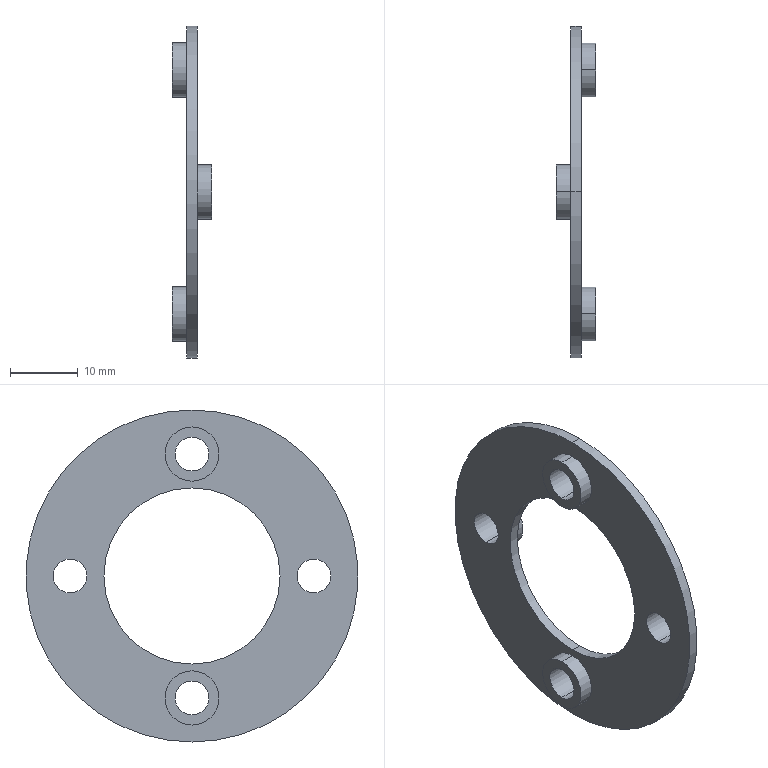Part | STEP file | _DBA01-D50-d20-e22-003 | 1 solid | 26 faces | box 5.9 x 49 x 49 mm | volume 2184 mm3 | cylinder 20 | plane 6 | commonest cylinder face diameters 5 x8 8 x8 26 x2 49 x2
STEP:
#1=CARTESIAN_POINT('',(-2.2,0.,14.));
#2=VERTEX_POINT('',#1);
#3=CARTESIAN_POINT('',(-2.2,0.,22.));
#4=VERTEX_POINT('',#3);
#5=CARTESIAN_POINT('',(-2.2,0.,18.));
#6=DIRECTION('',(-1.,0.,0.));
#7=DIRECTION('',(0.,0.,1.));
#8=AXIS2_PLACEMENT_3D('',#5,#6,#7);
#9=CIRCLE('',#8,4.);
#10=EDGE_CURVE('',#2,#4,#9,.T.);
#11=ORIENTED_EDGE('',*,*,#10,.F.);
#12=CARTESIAN_POINT('',(0.,0.,14.));
#13=VERTEX_POINT('',#12);
#14=CARTESIAN_POINT('',(-2.2,0.,14.));
#15=DIRECTION('',(1.,0.,0.));
#16=VECTOR('',#15,1000.);
#17=LINE('',#14,#16);
#18=EDGE_CURVE('',#2,#13,#17,.T.);
#19=ORIENTED_EDGE('',*,*,#18,.T.);
#20=CARTESIAN_POINT('',(0.,0.,22.));
#21=VERTEX_POINT('',#20);
#22=CARTESIAN_POINT('',(0.,0.,18.));
#23=DIRECTION('',(-1.,0.,0.));
#24=DIRECTION('',(0.,0.,1.));
#25=AXIS2_PLACEMENT_3D('',#22,#23,#24);
#26=CIRCLE('',#25,4.);
#27=EDGE_CURVE('',#13,#21,#26,.T.);
#28=ORIENTED_EDGE('',*,*,#27,.T.);
#29=CARTESIAN_POINT('',(-2.2,0.,22.));
#30=DIRECTION('',(1.,0.,0.));
#31=VECTOR('',#30,1000.);
#32=LINE('',#29,#31);
#33=EDGE_CURVE('',#4,#21,#32,.T.);
#34=ORIENTED_EDGE('',*,*,#33,.F.);
#35=EDGE_LOOP('',(#11,#19,#28,#34));
#36=FACE_OUTER_BOUND('',#35,.T.);
#37=CARTESIAN_POINT('',(-2.2,0.,18.));
#38=DIRECTION('',(1.,0.,0.));
#39=DIRECTION('',(0.,0.,1.));
#40=AXIS2_PLACEMENT_3D('',#37,#38,#39);
#41=CYLINDRICAL_SURFACE('',#40,4.);
#42=ADVANCED_FACE('',(#36),#41,.T.);
#43=CARTESIAN_POINT('',(-2.2,0.,-22.));
#44=VERTEX_POINT('',#43);
#45=CARTESIAN_POINT('',(-2.2,0.,-14.));
#46=VERTEX_POINT('',#45);
#47=CARTESIAN_POINT('',(-2.2,0.,-18.));
#48=DIRECTION('',(-1.,0.,0.));
#49=DIRECTION('',(0.,0.,1.));
#50=AXIS2_PLACEMENT_3D('',#47,#48,#49);
#51=CIRCLE('',#50,4.);
#52=EDGE_CURVE('',#44,#46,#51,.T.);
#53=ORIENTED_EDGE('',*,*,#52,.F.);
#54=CARTESIAN_POINT('',(0.,0.,-22.));
#55=VERTEX_POINT('',#54);
#56=CARTESIAN_POINT('',(-2.2,0.,-22.));
#57=DIRECTION('',(1.,0.,0.));
#58=VECTOR('',#57,1000.);
#59=LINE('',#56,#58);
#60=EDGE_CURVE('',#44,#55,#59,.T.);
#61=ORIENTED_EDGE('',*,*,#60,.T.);
#62=CARTESIAN_POINT('',(0.,0.,-14.));
#63=VERTEX_POINT('',#62);
#64=CARTESIAN_POINT('',(0.,0.,-18.));
#65=DIRECTION('',(-1.,0.,0.));
#66=DIRECTION('',(0.,0.,1.));
#67=AXIS2_PLACEMENT_3D('',#64,#65,#66);
#68=CIRCLE('',#67,4.);
#69=EDGE_CURVE('',#55,#63,#68,.T.);
#70=ORIENTED_EDGE('',*,*,#69,.T.);
#71=CARTESIAN_POINT('',(-2.2,0.,-14.));
#72=DIRECTION('',(1.,0.,0.));
#73=VECTOR('',#72,1000.);
#74=LINE('',#71,#73);
#75=EDGE_CURVE('',#46,#63,#74,.T.);
#76=ORIENTED_EDGE('',*,*,#75,.F.);
#77=EDGE_LOOP('',(#53,#61,#70,#76));
#78=FACE_OUTER_BOUND('',#77,.T.);
#79=CARTESIAN_POINT('',(-2.2,0.,-18.));
#80=DIRECTION('',(1.,0.,0.));
#81=DIRECTION('',(0.,0.,1.));
#82=AXIS2_PLACEMENT_3D('',#79,#80,#81);
#83=CYLINDRICAL_SURFACE('',#82,4.);
#84=ADVANCED_FACE('',(#78),#83,.T.);
#85=CARTESIAN_POINT('',(1.5,-18.,4.));
#86=VERTEX_POINT('',#85);
#87=CARTESIAN_POINT('',(1.5,-18.,-4.));
#88=VERTEX_POINT('',#87);
#89=CARTESIAN_POINT('',(1.5,-18.,0.));
#90=DIRECTION('',(1.,0.,0.));
#91=DIRECTION('',(0.,0.,-1.));
#92=AXIS2_PLACEMENT_3D('',#89,#90,#91);
#93=CIRCLE('',#92,4.);
#94=EDGE_CURVE('',#86,#88,#93,.T.);
#95=ORIENTED_EDGE('',*,*,#94,.T.);
#96=CARTESIAN_POINT('',(3.7,-18.,-4.));
#97=VERTEX_POINT('',#96);
#98=CARTESIAN_POINT('',(1.5,-18.,-4.));
#99=DIRECTION('',(1.,0.,0.));
#100=VECTOR('',#99,1000.);
#101=LINE('',#98,#100);
#102=EDGE_CURVE('',#88,#97,#101,.T.);
#103=ORIENTED_EDGE('',*,*,#102,.T.);
#104=CARTESIAN_POINT('',(3.7,-18.,4.));
#105=VERTEX_POINT('',#104);
#106=CARTESIAN_POINT('',(3.7,-18.,0.));
#107=DIRECTION('',(-1.,0.,0.));
#108=DIRECTION('',(0.,0.,1.));
#109=AXIS2_PLACEMENT_3D('',#106,#107,#108);
#110=CIRCLE('',#109,4.);
#111=EDGE_CURVE('',#97,#105,#110,.T.);
#112=ORIENTED_EDGE('',*,*,#111,.T.);
#113=CARTESIAN_POINT('',(1.5,-18.,4.));
#114=DIRECTION('',(1.,0.,0.));
#115=VECTOR('',#114,1000.);
#116=LINE('',#113,#115);
#117=EDGE_CURVE('',#86,#105,#116,.T.);
#118=ORIENTED_EDGE('',*,*,#117,.F.);
#119=EDGE_LOOP('',(#95,#103,#112,#118));
#120=FACE_OUTER_BOUND('',#119,.T.);
#121=CARTESIAN_POINT('',(1.5,-18.,0.));
#122=DIRECTION('',(1.,0.,0.));
#123=DIRECTION('',(0.,0.,1.));
#124=AXIS2_PLACEMENT_3D('',#121,#122,#123);
#125=CYLINDRICAL_SURFACE('',#124,4.);
#126=ADVANCED_FACE('',(#120),#125,.T.);
#127=CARTESIAN_POINT('',(1.5,18.,4.));
#128=VERTEX_POINT('',#127);
#129=CARTESIAN_POINT('',(1.5,18.,-4.));
#130=VERTEX_POINT('',#129);
#131=CARTESIAN_POINT('',(1.5,18.,0.));
#132=DIRECTION('',(1.,0.,0.));
#133=DIRECTION('',(0.,0.,-1.));
#134=AXIS2_PLACEMENT_3D('',#131,#132,#133);
#135=CIRCLE('',#134,4.);
#136=EDGE_CURVE('',#128,#130,#135,.T.);
#137=ORIENTED_EDGE('',*,*,#136,.T.);
#138=CARTESIAN_POINT('',(3.7,18.,-4.));
#139=VERTEX_POINT('',#138);
#140=CARTESIAN_POINT('',(1.5,18.,-4.));
#141=DIRECTION('',(1.,0.,0.));
#142=VECTOR('',#141,1000.);
#143=LINE('',#140,#142);
#144=EDGE_CURVE('',#130,#139,#143,.T.);
#145=ORIENTED_EDGE('',*,*,#144,.T.);
#146=CARTESIAN_POINT('',(3.7,18.,4.));
#147=VERTEX_POINT('',#146);
#148=CARTESIAN_POINT('',(3.7,18.,0.));
#149=DIRECTION('',(-1.,0.,0.));
#150=DIRECTION('',(0.,0.,1.));
#151=AXIS2_PLACEMENT_3D('',#148,#149,#150);
#152=CIRCLE('',#151,4.);
#153=EDGE_CURVE('',#139,#147,#152,.T.);
#154=ORIENTED_EDGE('',*,*,#153,.T.);
#155=CARTESIAN_POINT('',(1.5,18.,4.));
#156=DIRECTION('',(1.,0.,0.));
#157=VECTOR('',#156,1000.);
#158=LINE('',#155,#157);
#159=EDGE_CURVE('',#128,#147,#158,.T.);
#160=ORIENTED_EDGE('',*,*,#159,.F.);
#161=EDGE_LOOP('',(#137,#145,#154,#160));
#162=FACE_OUTER_BOUND('',#161,.T.);
#163=CARTESIAN_POINT('',(1.5,18.,0.));
#164=DIRECTION('',(1.,0.,0.));
#165=DIRECTION('',(0.,0.,1.));
#166=AXIS2_PLACEMENT_3D('',#163,#164,#165);
#167=CYLINDRICAL_SURFACE('',#166,4.);
#168=ADVANCED_FACE('',(#162),#167,.T.);
#169=CARTESIAN_POINT('',(-2.2,0.,-15.5));
#170=VERTEX_POINT('',#169);
#171=CARTESIAN_POINT('',(-2.2,0.,-20.5));
#172=VERTEX_POINT('',#171);
#173=CARTESIAN_POINT('',(-2.2,0.,-18.));
#174=DIRECTION('',(-1.,0.,0.));
#175=DIRECTION('',(0.,0.,1.));
#176=AXIS2_PLACEMENT_3D('',#173,#174,#175);
#177=CIRCLE('',#176,2.5);
#178=EDGE_CURVE('',#170,#172,#177,.T.);
#179=ORIENTED_EDGE('',*,*,#178,.T.);
#180=CARTESIAN_POINT('',(1.5,0.,-20.5));
#181=VERTEX_POINT('',#180);
#182=CARTESIAN_POINT('',(1.5,0.,-20.5));
#183=DIRECTION('',(1.,0.,0.));
#184=VECTOR('',#183,1000.);
#185=LINE('',#182,#184);
#186=EDGE_CURVE('',#172,#181,#185,.T.);
#187=ORIENTED_EDGE('',*,*,#186,.T.);
#188=CARTESIAN_POINT('',(1.5,0.,-15.5));
#189=VERTEX_POINT('',#188);
#190=CARTESIAN_POINT('',(1.5,0.,-18.));
#191=DIRECTION('',(1.,0.,0.));
#192=DIRECTION('',(0.,0.,-1.));
#193=AXIS2_PLACEMENT_3D('',#190,#191,#192);
#194=CIRCLE('',#193,2.5);
#195=EDGE_CURVE('',#181,#189,#194,.T.);
#196=ORIENTED_EDGE('',*,*,#195,.T.);
#197=CARTESIAN_POINT('',(1.5,0.,-15.5));
#198=DIRECTION('',(1.,0.,0.));
#199=VECTOR('',#198,1000.);
#200=LINE('',#197,#199);
#201=EDGE_CURVE('',#170,#189,#200,.T.);
#202=ORIENTED_EDGE('',*,*,#201,.F.);
#203=EDGE_LOOP('',(#179,#187,#196,#202));
#204=FACE_OUTER_BOUND('',#203,.T.);
#205=CARTESIAN_POINT('',(1.5,0.,-18.));
#206=DIRECTION('',(1.,0.,0.));
#207=DIRECTION('',(0.,0.,1.));
#208=AXIS2_PLACEMENT_3D('',#205,#206,#207);
#209=CYLINDRICAL_SURFACE('',#208,2.5);
#210=ADVANCED_FACE('',(#204),#209,.F.);
#211=CARTESIAN_POINT('',(0.,-18.,2.5));
#212=VERTEX_POINT('',#211);
#213=CARTESIAN_POINT('',(0.,-18.,-2.5));
#214=VERTEX_POINT('',#213);
#215=CARTESIAN_POINT('',(0.,-18.,0.));
#216=DIRECTION('',(-1.,0.,0.));
#217=DIRECTION('',(0.,0.,-1.));
#218=AXIS2_PLACEMENT_3D('',#215,#216,#217);
#219=CIRCLE('',#218,2.5);
#220=EDGE_CURVE('',#212,#214,#219,.T.);
#221=ORIENTED_EDGE('',*,*,#220,.T.);
#222=CARTESIAN_POINT('',(3.7,-18.,-2.5));
#223=VERTEX_POINT('',#222);
#224=CARTESIAN_POINT('',(1.5,-18.,-2.5));
#225=DIRECTION('',(1.,0.,0.));
#226=VECTOR('',#225,1000.);
#227=LINE('',#224,#226);
#228=EDGE_CURVE('',#214,#223,#227,.T.);
#229=ORIENTED_EDGE('',*,*,#228,.T.);
#230=CARTESIAN_POINT('',(3.7,-18.,2.5));
#231=VERTEX_POINT('',#230);
#232=CARTESIAN_POINT('',(3.7,-18.,0.));
#233=DIRECTION('',(-1.,0.,0.));
#234=DIRECTION('',(0.,0.,1.));
#235=AXIS2_PLACEMENT_3D('',#232,#233,#234);
#236=CIRCLE('',#235,2.5);
#237=EDGE_CURVE('',#231,#223,#236,.T.);
#238=ORIENTED_EDGE('',*,*,#237,.F.);
#239=CARTESIAN_POINT('',(1.5,-18.,2.5));
#240=DIRECTION('',(1.,0.,0.));
#241=VECTOR('',#240,1000.);
#242=LINE('',#239,#241);
#243=EDGE_CURVE('',#212,#231,#242,.T.);
#244=ORIENTED_EDGE('',*,*,#243,.F.);
#245=EDGE_LOOP('',(#221,#229,#238,#244));
#246=FACE_OUTER_BOUND('',#245,.T.);
#247=CARTESIAN_POINT('',(1.5,-18.,0.));
#248=DIRECTION('',(1.,0.,0.));
#249=DIRECTION('',(0.,0.,1.));
#250=AXIS2_PLACEMENT_3D('',#247,#248,#249);
#251=CYLINDRICAL_SURFACE('',#250,2.5);
#252=ADVANCED_FACE('',(#246),#251,.F.);
#253=CARTESIAN_POINT('',(-2.2,0.,20.5));
#254=VERTEX_POINT('',#253);
#255=CARTESIAN_POINT('',(-2.2,0.,15.5));
#256=VERTEX_POINT('',#255);
#257=CARTESIAN_POINT('',(-2.2,0.,18.));
#258=DIRECTION('',(-1.,0.,0.));
#259=DIRECTION('',(0.,0.,1.));
#260=AXIS2_PLACEMENT_3D('',#257,#258,#259);
#261=CIRCLE('',#260,2.5);
#262=EDGE_CURVE('',#254,#256,#261,.T.);
#263=ORIENTED_EDGE('',*,*,#262,.T.);
#264=CARTESIAN_POINT('',(1.5,0.,15.5));
#265=VERTEX_POINT('',#264);
#266=CARTESIAN_POINT('',(1.5,0.,15.5));
#267=DIRECTION('',(1.,0.,0.));
#268=VECTOR('',#267,1000.);
#269=LINE('',#266,#268);
#270=EDGE_CURVE('',#256,#265,#269,.T.);
#271=ORIENTED_EDGE('',*,*,#270,.T.);
#272=CARTESIAN_POINT('',(1.5,0.,20.5));
#273=VERTEX_POINT('',#272);
#274=CARTESIAN_POINT('',(1.5,0.,18.));
#275=DIRECTION('',(1.,0.,0.));
#276=DIRECTION('',(0.,0.,-1.));
#277=AXIS2_PLACEMENT_3D('',#274,#275,#276);
#278=CIRCLE('',#277,2.5);
#279=EDGE_CURVE('',#265,#273,#278,.T.);
#280=ORIENTED_EDGE('',*,*,#279,.T.);
#281=CARTESIAN_POINT('',(1.5,0.,20.5));
#282=DIRECTION('',(1.,0.,0.));
#283=VECTOR('',#282,1000.);
#284=LINE('',#281,#283);
#285=EDGE_CURVE('',#254,#273,#284,.T.);
#286=ORIENTED_EDGE('',*,*,#285,.F.);
#287=EDGE_LOOP('',(#263,#271,#280,#286));
#288=FACE_OUTER_BOUND('',#287,.T.);
#289=CARTESIAN_POINT('',(1.5,0.,18.));
#290=DIRECTION('',(1.,0.,0.));
#291=DIRECTION('',(0.,0.,1.));
#292=AXIS2_PLACEMENT_3D('',#289,#290,#291);
#293=CYLINDRICAL_SURFACE('',#292,2.5);
#294=ADVANCED_FACE('',(#288),#293,.F.);
#295=CARTESIAN_POINT('',(0.,18.,2.5));
#296=VERTEX_POINT('',#295);
#297=CARTESIAN_POINT('',(0.,18.,-2.5));
#298=VERTEX_POINT('',#297);
#299=CARTESIAN_POINT('',(0.,18.,0.));
#300=DIRECTION('',(-1.,0.,0.));
#301=DIRECTION('',(0.,0.,-1.));
#302=AXIS2_PLACEMENT_3D('',#299,#300,#301);
#303=CIRCLE('',#302,2.5);
#304=EDGE_CURVE('',#296,#298,#303,.T.);
#305=ORIENTED_EDGE('',*,*,#304,.T.);
#306=CARTESIAN_POINT('',(3.7,18.,-2.5));
#307=VERTEX_POINT('',#306);
#308=CARTESIAN_POINT('',(1.5,18.,-2.5));
#309=DIRECTION('',(1.,0.,0.));
#310=VECTOR('',#309,1000.);
#311=LINE('',#308,#310);
#312=EDGE_CURVE('',#298,#307,#311,.T.);
#313=ORIENTED_EDGE('',*,*,#312,.T.);
#314=CARTESIAN_POINT('',(3.7,18.,2.5));
#315=VERTEX_POINT('',#314);
#316=CARTESIAN_POINT('',(3.7,18.,0.));
#317=DIRECTION('',(-1.,0.,0.));
#318=DIRECTION('',(0.,0.,1.));
#319=AXIS2_PLACEMENT_3D('',#316,#317,#318);
#320=CIRCLE('',#319,2.5);
#321=EDGE_CURVE('',#315,#307,#320,.T.);
#322=ORIENTED_EDGE('',*,*,#321,.F.);
#323=CARTESIAN_POINT('',(1.5,18.,2.5));
#324=DIRECTION('',(1.,0.,0.));
#325=VECTOR('',#324,1000.);
#326=LINE('',#323,#325);
#327=EDGE_CURVE('',#296,#315,#326,.T.);
#328=ORIENTED_EDGE('',*,*,#327,.F.);
#329=EDGE_LOOP('',(#305,#313,#322,#328));
#330=FACE_OUTER_BOUND('',#329,.T.);
#331=CARTESIAN_POINT('',(1.5,18.,0.));
#332=DIRECTION('',(1.,0.,0.));
#333=DIRECTION('',(0.,0.,1.));
#334=AXIS2_PLACEMENT_3D('',#331,#332,#333);
#335=CYLINDRICAL_SURFACE('',#334,2.5);
#336=ADVANCED_FACE('',(#330),#335,.F.);
#337=CARTESIAN_POINT('',(0.,0.,-13.));
#338=VERTEX_POINT('',#337);
#339=CARTESIAN_POINT('',(0.,0.,13.));
#340=VERTEX_POINT('',#339);
#341=CARTESIAN_POINT('',(0.,0.,0.));
#342=DIRECTION('',(1.,0.,0.));
#343=DIRECTION('',(0.,0.,-1.));
#344=AXIS2_PLACEMENT_3D('',#341,#342,#343);
#345=CIRCLE('',#344,13.);
#346=EDGE_CURVE('',#338,#340,#345,.T.);
#347=ORIENTED_EDGE('',*,*,#346,.F.);
#348=CARTESIAN_POINT('',(1.5,0.,-13.));
#349=VERTEX_POINT('',#348);
#350=CARTESIAN_POINT('',(1.5,0.,-13.));
#351=DIRECTION('',(1.,0.,0.));
#352=VECTOR('',#351,1000.);
#353=LINE('',#350,#352);
#354=EDGE_CURVE('',#338,#349,#353,.T.);
#355=ORIENTED_EDGE('',*,*,#354,.T.);
#356=CARTESIAN_POINT('',(1.5,0.,13.));
#357=VERTEX_POINT('',#356);
#358=CARTESIAN_POINT('',(1.5,0.,0.));
#359=DIRECTION('',(1.,0.,0.));
#360=DIRECTION('',(0.,0.,-1.));
#361=AXIS2_PLACEMENT_3D('',#358,#359,#360);
#362=CIRCLE('',#361,13.);
#363=EDGE_CURVE('',#349,#357,#362,.T.);
#364=ORIENTED_EDGE('',*,*,#363,.T.);
#365=CARTESIAN_POINT('',(1.5,0.,13.));
#366=DIRECTION('',(1.,0.,0.));
#367=VECTOR('',#366,1000.);
#368=LINE('',#365,#367);
#369=EDGE_CURVE('',#340,#357,#368,.T.);
#370=ORIENTED_EDGE('',*,*,#369,.F.);
#371=EDGE_LOOP('',(#347,#355,#364,#370));
#372=FACE_OUTER_BOUND('',#371,.T.);
#373=CARTESIAN_POINT('',(1.5,0.,0.));
#374=DIRECTION('',(1.,0.,0.));
#375=DIRECTION('',(0.,0.,1.));
#376=AXIS2_PLACEMENT_3D('',#373,#374,#375);
#377=CYLINDRICAL_SURFACE('',#376,13.);
#378=ADVANCED_FACE('',(#372),#377,.F.);
#379=CARTESIAN_POINT('',(0.,0.,24.5));
#380=VERTEX_POINT('',#379);
#381=CARTESIAN_POINT('',(0.,0.,-24.5));
#382=VERTEX_POINT('',#381);
#383=CARTESIAN_POINT('',(0.,0.,0.));
#384=DIRECTION('',(1.,0.,0.));
#385=DIRECTION('',(0.,0.,-1.));
#386=AXIS2_PLACEMENT_3D('',#383,#384,#385);
#387=CIRCLE('',#386,24.5);
#388=EDGE_CURVE('',#380,#382,#387,.T.);
#389=ORIENTED_EDGE('',*,*,#388,.T.);
#390=CARTESIAN_POINT('',(1.5,0.,-24.5));
#391=VERTEX_POINT('',#390);
#392=CARTESIAN_POINT('',(1.5,0.,-24.5));
#393=DIRECTION('',(1.,0.,0.));
#394=VECTOR('',#393,1000.);
#395=LINE('',#392,#394);
#396=EDGE_CURVE('',#382,#391,#395,.T.);
#397=ORIENTED_EDGE('',*,*,#396,.T.);
#398=CARTESIAN_POINT('',(1.5,0.,24.5));
#399=VERTEX_POINT('',#398);
#400=CARTESIAN_POINT('',(1.5,0.,0.));
#401=DIRECTION('',(1.,0.,0.));
#402=DIRECTION('',(0.,0.,-1.));
#403=AXIS2_PLACEMENT_3D('',#400,#401,#402);
#404=CIRCLE('',#403,24.5);
#405=EDGE_CURVE('',#399,#391,#404,.T.);
#406=ORIENTED_EDGE('',*,*,#405,.F.);
#407=CARTESIAN_POINT('',(1.5,0.,24.5));
#408=DIRECTION('',(1.,0.,0.));
#409=VECTOR('',#408,1000.);
#410=LINE('',#407,#409);
#411=EDGE_CURVE('',#380,#399,#410,.T.);
#412=ORIENTED_EDGE('',*,*,#411,.F.);
#413=EDGE_LOOP('',(#389,#397,#406,#412));
#414=FACE_OUTER_BOUND('',#413,.T.);
#415=CARTESIAN_POINT('',(1.5,0.,0.));
#416=DIRECTION('',(1.,0.,0.));
#417=DIRECTION('',(0.,0.,1.));
#418=AXIS2_PLACEMENT_3D('',#415,#416,#417);
#419=CYLINDRICAL_SURFACE('',#418,24.5);
#420=ADVANCED_FACE('',(#414),#419,.T.);
#421=ORIENTED_EDGE('',*,*,#388,.F.);
#422=CARTESIAN_POINT('',(0.,0.,0.));
#423=DIRECTION('',(1.,0.,0.));
#424=DIRECTION('',(0.,0.,-1.));
#425=AXIS2_PLACEMENT_3D('',#422,#423,#424);
#426=CIRCLE('',#425,24.5);
#427=EDGE_CURVE('',#382,#380,#426,.T.);
#428=ORIENTED_EDGE('',*,*,#427,.F.);
#429=EDGE_LOOP('',(#421,#428));
#430=FACE_OUTER_BOUND('',#429,.T.);
#431=CARTESIAN_POINT('',(0.,0.,18.));
#432=DIRECTION('',(-1.,0.,0.));
#433=DIRECTION('',(0.,0.,1.));
#434=AXIS2_PLACEMENT_3D('',#431,#432,#433);
#435=CIRCLE('',#434,4.);
#436=EDGE_CURVE('',#21,#13,#435,.T.);
#437=ORIENTED_EDGE('',*,*,#436,.F.);
#438=ORIENTED_EDGE('',*,*,#27,.F.);
#439=EDGE_LOOP('',(#437,#438));
#440=FACE_BOUND('',#439,.T.);
#441=CARTESIAN_POINT('',(0.,0.,-18.));
#442=DIRECTION('',(-1.,0.,0.));
#443=DIRECTION('',(0.,0.,1.));
#444=AXIS2_PLACEMENT_3D('',#441,#442,#443);
#445=CIRCLE('',#444,4.);
#446=EDGE_CURVE('',#63,#55,#445,.T.);
#447=ORIENTED_EDGE('',*,*,#446,.F.);
#448=ORIENTED_EDGE('',*,*,#69,.F.);
#449=EDGE_LOOP('',(#447,#448));
#450=FACE_BOUND('',#449,.T.);
#451=ORIENTED_EDGE('',*,*,#220,.F.);
#452=CARTESIAN_POINT('',(0.,-18.,0.));
#453=DIRECTION('',(-1.,0.,0.));
#454=DIRECTION('',(0.,0.,-1.));
#455=AXIS2_PLACEMENT_3D('',#452,#453,#454);
#456=CIRCLE('',#455,2.5);
#457=EDGE_CURVE('',#214,#212,#456,.T.);
#458=ORIENTED_EDGE('',*,*,#457,.F.);
#459=EDGE_LOOP('',(#451,#458));
#460=FACE_BOUND('',#459,.T.);
#461=ORIENTED_EDGE('',*,*,#304,.F.);
#462=CARTESIAN_POINT('',(0.,18.,0.));
#463=DIRECTION('',(-1.,0.,0.));
#464=DIRECTION('',(0.,0.,-1.));
#465=AXIS2_PLACEMENT_3D('',#462,#463,#464);
#466=CIRCLE('',#465,2.5);
#467=EDGE_CURVE('',#298,#296,#466,.T.);
#468=ORIENTED_EDGE('',*,*,#467,.F.);
#469=EDGE_LOOP('',(#461,#468));
#470=FACE_BOUND('',#469,.T.);
#471=CARTESIAN_POINT('',(0.,0.,0.));
#472=DIRECTION('',(1.,0.,0.));
#473=DIRECTION('',(0.,0.,-1.));
#474=AXIS2_PLACEMENT_3D('',#471,#472,#473);
#475=CIRCLE('',#474,13.);
#476=EDGE_CURVE('',#340,#338,#475,.T.);
#477=ORIENTED_EDGE('',*,*,#476,.T.);
#478=ORIENTED_EDGE('',*,*,#346,.T.);
#479=EDGE_LOOP('',(#477,#478));
#480=FACE_BOUND('',#479,.T.);
#481=CARTESIAN_POINT('',(0.,0.,0.));
#482=DIRECTION('',(1.,0.,0.));
#483=DIRECTION('',(0.,1.,0.));
#484=AXIS2_PLACEMENT_3D('',#481,#482,#483);
#485=PLANE('',#484);
#486=ADVANCED_FACE('',(#430,#440,#450,#460,#470,#480),#485,.F.);
#487=ORIENTED_EDGE('',*,*,#396,.F.);
#488=ORIENTED_EDGE('',*,*,#427,.T.);
#489=ORIENTED_EDGE('',*,*,#411,.T.);
#490=CARTESIAN_POINT('',(1.5,0.,0.));
#491=DIRECTION('',(1.,0.,0.));
#492=DIRECTION('',(0.,0.,-1.));
#493=AXIS2_PLACEMENT_3D('',#490,#491,#492);
#494=CIRCLE('',#493,24.5);
#495=EDGE_CURVE('',#391,#399,#494,.T.);
#496=ORIENTED_EDGE('',*,*,#495,.F.);
#497=EDGE_LOOP('',(#487,#488,#489,#496));
#498=FACE_OUTER_BOUND('',#497,.T.);
#499=CARTESIAN_POINT('',(1.5,0.,0.));
#500=DIRECTION('',(1.,0.,0.));
#501=DIRECTION('',(0.,0.,1.));
#502=AXIS2_PLACEMENT_3D('',#499,#500,#501);
#503=CYLINDRICAL_SURFACE('',#502,24.5);
#504=ADVANCED_FACE('',(#498),#503,.T.);
#505=ORIENTED_EDGE('',*,*,#405,.T.);
#506=ORIENTED_EDGE('',*,*,#495,.T.);
#507=EDGE_LOOP('',(#505,#506));
#508=FACE_OUTER_BOUND('',#507,.T.);
#509=ORIENTED_EDGE('',*,*,#94,.F.);
#510=CARTESIAN_POINT('',(1.5,-18.,0.));
#511=DIRECTION('',(1.,0.,0.));
#512=DIRECTION('',(0.,0.,-1.));
#513=AXIS2_PLACEMENT_3D('',#510,#511,#512);
#514=CIRCLE('',#513,4.);
#515=EDGE_CURVE('',#88,#86,#514,.T.);
#516=ORIENTED_EDGE('',*,*,#515,.F.);
#517=EDGE_LOOP('',(#509,#516));
#518=FACE_BOUND('',#517,.T.);
#519=ORIENTED_EDGE('',*,*,#136,.F.);
#520=CARTESIAN_POINT('',(1.5,18.,0.));
#521=DIRECTION('',(1.,0.,0.));
#522=DIRECTION('',(0.,0.,-1.));
#523=AXIS2_PLACEMENT_3D('',#520,#521,#522);
#524=CIRCLE('',#523,4.);
#525=EDGE_CURVE('',#130,#128,#524,.T.);
#526=ORIENTED_EDGE('',*,*,#525,.F.);
#527=EDGE_LOOP('',(#519,#526));
#528=FACE_BOUND('',#527,.T.);
#529=CARTESIAN_POINT('',(1.5,0.,-18.));
#530=DIRECTION('',(1.,0.,0.));
#531=DIRECTION('',(0.,0.,-1.));
#532=AXIS2_PLACEMENT_3D('',#529,#530,#531);
#533=CIRCLE('',#532,2.5);
#534=EDGE_CURVE('',#189,#181,#533,.T.);
#535=ORIENTED_EDGE('',*,*,#534,.F.);
#536=ORIENTED_EDGE('',*,*,#195,.F.);
#537=EDGE_LOOP('',(#535,#536));
#538=FACE_BOUND('',#537,.T.);
#539=CARTESIAN_POINT('',(1.5,0.,18.));
#540=DIRECTION('',(1.,0.,0.));
#541=DIRECTION('',(0.,0.,-1.));
#542=AXIS2_PLACEMENT_3D('',#539,#540,#541);
#543=CIRCLE('',#542,2.5);
#544=EDGE_CURVE('',#273,#265,#543,.T.);
#545=ORIENTED_EDGE('',*,*,#544,.F.);
#546=ORIENTED_EDGE('',*,*,#279,.F.);
#547=EDGE_LOOP('',(#545,#546));
#548=FACE_BOUND('',#547,.T.);
#549=CARTESIAN_POINT('',(1.5,0.,0.));
#550=DIRECTION('',(1.,0.,0.));
#551=DIRECTION('',(0.,0.,-1.));
#552=AXIS2_PLACEMENT_3D('',#549,#550,#551);
#553=CIRCLE('',#552,13.);
#554=EDGE_CURVE('',#357,#349,#553,.T.);
#555=ORIENTED_EDGE('',*,*,#554,.F.);
#556=ORIENTED_EDGE('',*,*,#363,.F.);
#557=EDGE_LOOP('',(#555,#556));
#558=FACE_BOUND('',#557,.T.);
#559=CARTESIAN_POINT('',(1.5,0.,0.));
#560=DIRECTION('',(1.,0.,0.));
#561=DIRECTION('',(0.,1.,0.));
#562=AXIS2_PLACEMENT_3D('',#559,#560,#561);
#563=PLANE('',#562);
#564=ADVANCED_FACE('',(#508,#518,#528,#538,#548,#558),#563,.T.);
#565=ORIENTED_EDGE('',*,*,#354,.F.);
#566=ORIENTED_EDGE('',*,*,#476,.F.);
#567=ORIENTED_EDGE('',*,*,#369,.T.);
#568=ORIENTED_EDGE('',*,*,#554,.T.);
#569=EDGE_LOOP('',(#565,#566,#567,#568));
#570=FACE_OUTER_BOUND('',#569,.T.);
#571=CARTESIAN_POINT('',(1.5,0.,0.));
#572=DIRECTION('',(1.,0.,0.));
#573=DIRECTION('',(0.,0.,1.));
#574=AXIS2_PLACEMENT_3D('',#571,#572,#573);
#575=CYLINDRICAL_SURFACE('',#574,13.);
#576=ADVANCED_FACE('',(#570),#575,.F.);
#577=ORIENTED_EDGE('',*,*,#312,.F.);
#578=ORIENTED_EDGE('',*,*,#467,.T.);
#579=ORIENTED_EDGE('',*,*,#327,.T.);
#580=CARTESIAN_POINT('',(3.7,18.,0.));
#581=DIRECTION('',(-1.,0.,0.));
#582=DIRECTION('',(0.,0.,1.));
#583=AXIS2_PLACEMENT_3D('',#580,#581,#582);
#584=CIRCLE('',#583,2.5);
#585=EDGE_CURVE('',#307,#315,#584,.T.);
#586=ORIENTED_EDGE('',*,*,#585,.F.);
#587=EDGE_LOOP('',(#577,#578,#579,#586));
#588=FACE_OUTER_BOUND('',#587,.T.);
#589=CARTESIAN_POINT('',(1.5,18.,0.));
#590=DIRECTION('',(1.,0.,0.));
#591=DIRECTION('',(0.,0.,1.));
#592=AXIS2_PLACEMENT_3D('',#589,#590,#591);
#593=CYLINDRICAL_SURFACE('',#592,2.5);
#594=ADVANCED_FACE('',(#588),#593,.F.);
#595=ORIENTED_EDGE('',*,*,#270,.F.);
#596=CARTESIAN_POINT('',(-2.2,0.,18.));
#597=DIRECTION('',(-1.,0.,0.));
#598=DIRECTION('',(0.,0.,1.));
#599=AXIS2_PLACEMENT_3D('',#596,#597,#598);
#600=CIRCLE('',#599,2.5);
#601=EDGE_CURVE('',#256,#254,#600,.T.);
#602=ORIENTED_EDGE('',*,*,#601,.T.);
#603=ORIENTED_EDGE('',*,*,#285,.T.);
#604=ORIENTED_EDGE('',*,*,#544,.T.);
#605=EDGE_LOOP('',(#595,#602,#603,#604));
#606=FACE_OUTER_BOUND('',#605,.T.);
#607=CARTESIAN_POINT('',(1.5,0.,18.));
#608=DIRECTION('',(1.,0.,0.));
#609=DIRECTION('',(0.,0.,1.));
#610=AXIS2_PLACEMENT_3D('',#607,#608,#609);
#611=CYLINDRICAL_SURFACE('',#610,2.5);
#612=ADVANCED_FACE('',(#606),#611,.F.);
#613=ORIENTED_EDGE('',*,*,#228,.F.);
#614=ORIENTED_EDGE('',*,*,#457,.T.);
#615=ORIENTED_EDGE('',*,*,#243,.T.);
#616=CARTESIAN_POINT('',(3.7,-18.,0.));
#617=DIRECTION('',(-1.,0.,0.));
#618=DIRECTION('',(0.,0.,1.));
#619=AXIS2_PLACEMENT_3D('',#616,#617,#618);
#620=CIRCLE('',#619,2.5);
#621=EDGE_CURVE('',#223,#231,#620,.T.);
#622=ORIENTED_EDGE('',*,*,#621,.F.);
#623=EDGE_LOOP('',(#613,#614,#615,#622));
#624=FACE_OUTER_BOUND('',#623,.T.);
#625=CARTESIAN_POINT('',(1.5,-18.,0.));
#626=DIRECTION('',(1.,0.,0.));
#627=DIRECTION('',(0.,0.,1.));
#628=AXIS2_PLACEMENT_3D('',#625,#626,#627);
#629=CYLINDRICAL_SURFACE('',#628,2.5);
#630=ADVANCED_FACE('',(#624),#629,.F.);
#631=ORIENTED_EDGE('',*,*,#186,.F.);
#632=CARTESIAN_POINT('',(-2.2,0.,-18.));
#633=DIRECTION('',(-1.,0.,0.));
#634=DIRECTION('',(0.,0.,1.));
#635=AXIS2_PLACEMENT_3D('',#632,#633,#634);
#636=CIRCLE('',#635,2.5);
#637=EDGE_CURVE('',#172,#170,#636,.T.);
#638=ORIENTED_EDGE('',*,*,#637,.T.);
#639=ORIENTED_EDGE('',*,*,#201,.T.);
#640=ORIENTED_EDGE('',*,*,#534,.T.);
#641=EDGE_LOOP('',(#631,#638,#639,#640));
#642=FACE_OUTER_BOUND('',#641,.T.);
#643=CARTESIAN_POINT('',(1.5,0.,-18.));
#644=DIRECTION('',(1.,0.,0.));
#645=DIRECTION('',(0.,0.,1.));
#646=AXIS2_PLACEMENT_3D('',#643,#644,#645);
#647=CYLINDRICAL_SURFACE('',#646,2.5);
#648=ADVANCED_FACE('',(#642),#647,.F.);
#649=ORIENTED_EDGE('',*,*,#144,.F.);
#650=ORIENTED_EDGE('',*,*,#525,.T.);
#651=ORIENTED_EDGE('',*,*,#159,.T.);
#652=CARTESIAN_POINT('',(3.7,18.,0.));
#653=DIRECTION('',(-1.,0.,0.));
#654=DIRECTION('',(0.,0.,1.));
#655=AXIS2_PLACEMENT_3D('',#652,#653,#654);
#656=CIRCLE('',#655,4.);
#657=EDGE_CURVE('',#147,#139,#656,.T.);
#658=ORIENTED_EDGE('',*,*,#657,.T.);
#659=EDGE_LOOP('',(#649,#650,#651,#658));
#660=FACE_OUTER_BOUND('',#659,.T.);
#661=CARTESIAN_POINT('',(1.5,18.,0.));
#662=DIRECTION('',(1.,0.,0.));
#663=DIRECTION('',(0.,0.,1.));
#664=AXIS2_PLACEMENT_3D('',#661,#662,#663);
#665=CYLINDRICAL_SURFACE('',#664,4.);
#666=ADVANCED_FACE('',(#660),#665,.T.);
#667=ORIENTED_EDGE('',*,*,#657,.F.);
#668=ORIENTED_EDGE('',*,*,#153,.F.);
#669=EDGE_LOOP('',(#667,#668));
#670=FACE_OUTER_BOUND('',#669,.T.);
#671=ORIENTED_EDGE('',*,*,#321,.T.);
#672=ORIENTED_EDGE('',*,*,#585,.T.);
#673=EDGE_LOOP('',(#671,#672));
#674=FACE_BOUND('',#673,.T.);
#675=CARTESIAN_POINT('',(3.7,14.,0.));
#676=DIRECTION('',(1.,0.,0.));
#677=DIRECTION('',(0.,1.,0.));
#678=AXIS2_PLACEMENT_3D('',#675,#676,#677);
#679=PLANE('',#678);
#680=ADVANCED_FACE('',(#670,#674),#679,.T.);
#681=ORIENTED_EDGE('',*,*,#102,.F.);
#682=ORIENTED_EDGE('',*,*,#515,.T.);
#683=ORIENTED_EDGE('',*,*,#117,.T.);
#684=CARTESIAN_POINT('',(3.7,-18.,0.));
#685=DIRECTION('',(-1.,0.,0.));
#686=DIRECTION('',(0.,0.,1.));
#687=AXIS2_PLACEMENT_3D('',#684,#685,#686);
#688=CIRCLE('',#687,4.);
#689=EDGE_CURVE('',#105,#97,#688,.T.);
#690=ORIENTED_EDGE('',*,*,#689,.T.);
#691=EDGE_LOOP('',(#681,#682,#683,#690));
#692=FACE_OUTER_BOUND('',#691,.T.);
#693=CARTESIAN_POINT('',(1.5,-18.,0.));
#694=DIRECTION('',(1.,0.,0.));
#695=DIRECTION('',(0.,0.,1.));
#696=AXIS2_PLACEMENT_3D('',#693,#694,#695);
#697=CYLINDRICAL_SURFACE('',#696,4.);
#698=ADVANCED_FACE('',(#692),#697,.T.);
#699=ORIENTED_EDGE('',*,*,#689,.F.);
#700=ORIENTED_EDGE('',*,*,#111,.F.);
#701=EDGE_LOOP('',(#699,#700));
#702=FACE_OUTER_BOUND('',#701,.T.);
#703=ORIENTED_EDGE('',*,*,#237,.T.);
#704=ORIENTED_EDGE('',*,*,#621,.T.);
#705=EDGE_LOOP('',(#703,#704));
#706=FACE_BOUND('',#705,.T.);
#707=CARTESIAN_POINT('',(3.7,-22.,0.));
#708=DIRECTION('',(1.,0.,0.));
#709=DIRECTION('',(0.,1.,0.));
#710=AXIS2_PLACEMENT_3D('',#707,#708,#709);
#711=PLANE('',#710);
#712=ADVANCED_FACE('',(#702,#706),#711,.T.);
#713=CARTESIAN_POINT('',(-2.2,0.,-18.));
#714=DIRECTION('',(-1.,0.,0.));
#715=DIRECTION('',(0.,0.,1.));
#716=AXIS2_PLACEMENT_3D('',#713,#714,#715);
#717=CIRCLE('',#716,4.);
#718=EDGE_CURVE('',#46,#44,#717,.T.);
#719=ORIENTED_EDGE('',*,*,#718,.T.);
#720=ORIENTED_EDGE('',*,*,#52,.T.);
#721=EDGE_LOOP('',(#719,#720));
#722=FACE_OUTER_BOUND('',#721,.T.);
#723=ORIENTED_EDGE('',*,*,#178,.F.);
#724=ORIENTED_EDGE('',*,*,#637,.F.);
#725=EDGE_LOOP('',(#723,#724));
#726=FACE_BOUND('',#725,.T.);
#727=CARTESIAN_POINT('',(-2.2,0.,-15.5));
#728=DIRECTION('',(-1.,0.,0.));
#729=DIRECTION('',(0.,0.,1.));
#730=AXIS2_PLACEMENT_3D('',#727,#728,#729);
#731=PLANE('',#730);
#732=ADVANCED_FACE('',(#722,#726),#731,.T.);
#733=ORIENTED_EDGE('',*,*,#60,.F.);
#734=ORIENTED_EDGE('',*,*,#718,.F.);
#735=ORIENTED_EDGE('',*,*,#75,.T.);
#736=ORIENTED_EDGE('',*,*,#446,.T.);
#737=EDGE_LOOP('',(#733,#734,#735,#736));
#738=FACE_OUTER_BOUND('',#737,.T.);
#739=CARTESIAN_POINT('',(-2.2,0.,-18.));
#740=DIRECTION('',(1.,0.,0.));
#741=DIRECTION('',(0.,0.,1.));
#742=AXIS2_PLACEMENT_3D('',#739,#740,#741);
#743=CYLINDRICAL_SURFACE('',#742,4.);
#744=ADVANCED_FACE('',(#738),#743,.T.);
#745=CARTESIAN_POINT('',(-2.2,0.,18.));
#746=DIRECTION('',(-1.,0.,0.));
#747=DIRECTION('',(0.,0.,1.));
#748=AXIS2_PLACEMENT_3D('',#745,#746,#747);
#749=CIRCLE('',#748,4.);
#750=EDGE_CURVE('',#4,#2,#749,.T.);
#751=ORIENTED_EDGE('',*,*,#750,.T.);
#752=ORIENTED_EDGE('',*,*,#10,.T.);
#753=EDGE_LOOP('',(#751,#752));
#754=FACE_OUTER_BOUND('',#753,.T.);
#755=ORIENTED_EDGE('',*,*,#262,.F.);
#756=ORIENTED_EDGE('',*,*,#601,.F.);
#757=EDGE_LOOP('',(#755,#756));
#758=FACE_BOUND('',#757,.T.);
#759=CARTESIAN_POINT('',(-2.2,0.,20.5));
#760=DIRECTION('',(-1.,0.,0.));
#761=DIRECTION('',(0.,0.,1.));
#762=AXIS2_PLACEMENT_3D('',#759,#760,#761);
#763=PLANE('',#762);
#764=ADVANCED_FACE('',(#754,#758),#763,.T.);
#765=ORIENTED_EDGE('',*,*,#18,.F.);
#766=ORIENTED_EDGE('',*,*,#750,.F.);
#767=ORIENTED_EDGE('',*,*,#33,.T.);
#768=ORIENTED_EDGE('',*,*,#436,.T.);
#769=EDGE_LOOP('',(#765,#766,#767,#768));
#770=FACE_OUTER_BOUND('',#769,.T.);
#771=CARTESIAN_POINT('',(-2.2,0.,18.));
#772=DIRECTION('',(1.,0.,0.));
#773=DIRECTION('',(0.,0.,1.));
#774=AXIS2_PLACEMENT_3D('',#771,#772,#773);
#775=CYLINDRICAL_SURFACE('',#774,4.);
#776=ADVANCED_FACE('',(#770),#775,.T.);
#777=CLOSED_SHELL('',(#42,#84,#126,#168,#210,#252,#294,#336,#378,#420,#486,#504,#564,#576,#594,#612,#630,#648,#666,#680,#698,#712,#732,#744,#764,#776));
#778=MANIFOLD_SOLID_BREP('',#777);
#779=CARTESIAN_POINT('',(0.,0.,0.));
#780=DIRECTION('',(0.,0.,1.));
#781=DIRECTION('',(1.,0.,0.));
#782=AXIS2_PLACEMENT_3D('',#779,#780,#781);
#783=(LENGTH_UNIT()NAMED_UNIT(*)SI_UNIT(.MILLI.,.METRE.));
#784=UNCERTAINTY_MEASURE_WITH_UNIT(LENGTH_MEASURE(0.00001),#783,'','');
#785=(NAMED_UNIT(*)PLANE_ANGLE_UNIT()SI_UNIT($,.RADIAN.));
#786=(NAMED_UNIT(*)SI_UNIT($,.STERADIAN.)SOLID_ANGLE_UNIT());
#787=(GEOMETRIC_REPRESENTATION_CONTEXT(3)GLOBAL_UNCERTAINTY_ASSIGNED_CONTEXT((#784))GLOBAL_UNIT_ASSIGNED_CONTEXT((#783,#785,#786))REPRESENTATION_CONTEXT('',''));
#788=ADVANCED_BREP_SHAPE_REPRESENTATION('',(#778,#782),#787);